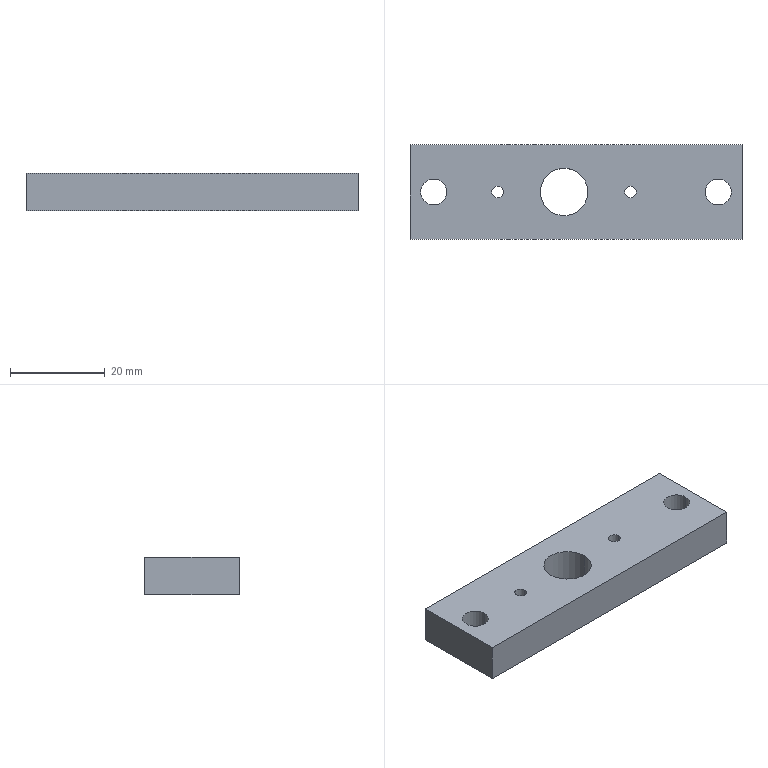Part | STEP file | positioning cylinder plate | 1 solid | 16 faces | box 70 x 20 x 8 mm | volume 10113 mm3 | cylinder 10 | plane 6 | commonest cylinder face diameters 2.5 x4 5.5 x4 10 x2
STEP:
#1=CARTESIAN_POINT('',(0.,0.,0.));
#2=DIRECTION('',(0.,0.,1.));
#3=DIRECTION('',(1.,0.,0.));
#4=AXIS2_PLACEMENT_3D('',#1,#2,#3);
#5=CARTESIAN_POINT('',(-12.75,0.,0.));
#6=VERTEX_POINT('',#5);
#7=CARTESIAN_POINT('',(-12.75,0.,8.));
#8=VERTEX_POINT('',#7);
#9=CARTESIAN_POINT('',(-12.75,0.,8.));
#10=DIRECTION('',(0.,0.,1.));
#11=VECTOR('',#10,1.);
#12=LINE('',#9,#11);
#13=CARTESIAN_POINT('',(-14.,0.,8.));
#14=DIRECTION('',(0.,0.,1.));
#15=DIRECTION('',(1.,0.,0.));
#16=AXIS2_PLACEMENT_3D('',#13,#14,#15);
#17=CYLINDRICAL_SURFACE('',#16,1.25);
#18=CARTESIAN_POINT('',(6.283,0.));
#19=DIRECTION('',(0.,1.));
#20=VECTOR('',#19,1.);
#21=LINE('',#18,#20);
#22=(GEOMETRIC_REPRESENTATION_CONTEXT(2)PARAMETRIC_REPRESENTATION_CONTEXT()REPRESENTATION_CONTEXT('',''));
#23=DEFINITIONAL_REPRESENTATION('',(#21),#22);
#24=PCURVE('',#17,#23);
#25=CARTESIAN_POINT('',(-14.,0.,8.));
#26=DIRECTION('',(0.,0.,1.));
#27=DIRECTION('',(1.,0.,0.));
#28=AXIS2_PLACEMENT_3D('',#25,#26,#27);
#29=CYLINDRICAL_SURFACE('',#28,1.25);
#30=CARTESIAN_POINT('',(0.,0.));
#31=DIRECTION('',(0.,1.));
#32=VECTOR('',#31,1.);
#33=LINE('',#30,#32);
#34=(GEOMETRIC_REPRESENTATION_CONTEXT(2)PARAMETRIC_REPRESENTATION_CONTEXT()REPRESENTATION_CONTEXT('',''));
#35=DEFINITIONAL_REPRESENTATION('',(#33),#34);
#36=PCURVE('',#29,#35);
#37=SURFACE_CURVE('',#12,(#24,#36),.PCURVE_S1.);
#38=EDGE_CURVE('',#6,#8,#37,.T.);
#39=ORIENTED_EDGE('',*,*,#38,.T.);
#40=CARTESIAN_POINT('',(-15.25,0.,8.));
#41=VERTEX_POINT('',#40);
#42=CARTESIAN_POINT('',(-14.,0.,8.));
#43=DIRECTION('',(0.,0.,1.));
#44=DIRECTION('',(1.,0.,0.));
#45=AXIS2_PLACEMENT_3D('',#42,#43,#44);
#46=CIRCLE('',#45,1.25);
#47=CARTESIAN_POINT('',(0.,0.));
#48=DIRECTION('',(1.,0.));
#49=VECTOR('',#48,1.);
#50=LINE('',#47,#49);
#51=(GEOMETRIC_REPRESENTATION_CONTEXT(2)PARAMETRIC_REPRESENTATION_CONTEXT()REPRESENTATION_CONTEXT('',''));
#52=DEFINITIONAL_REPRESENTATION('',(#50),#51);
#53=PCURVE('',#17,#52);
#54=CARTESIAN_POINT('',(37.5,-10.,8.));
#55=DIRECTION('',(0.,0.,1.));
#56=DIRECTION('',(1.,0.,0.));
#57=AXIS2_PLACEMENT_3D('',#54,#55,#56);
#58=PLANE('',#57);
#59=CARTESIAN_POINT('',(-51.5,10.));
#60=DIRECTION('',(1.,0.));
#61=AXIS2_PLACEMENT_2D('',#59,#60);
#62=CIRCLE('',#61,1.25);
#63=(GEOMETRIC_REPRESENTATION_CONTEXT(2)PARAMETRIC_REPRESENTATION_CONTEXT()REPRESENTATION_CONTEXT('',''));
#64=DEFINITIONAL_REPRESENTATION('',(#62),#63);
#65=PCURVE('',#58,#64);
#66=SURFACE_CURVE('',#46,(#53,#65),.PCURVE_S1.);
#67=EDGE_CURVE('',#41,#8,#66,.T.);
#68=ORIENTED_EDGE('',*,*,#67,.F.);
#69=CARTESIAN_POINT('',(-15.25,0.,0.));
#70=VERTEX_POINT('',#69);
#71=CARTESIAN_POINT('',(-15.25,0.,8.));
#72=DIRECTION('',(0.,0.,1.));
#73=VECTOR('',#72,1.);
#74=LINE('',#71,#73);
#75=CARTESIAN_POINT('',(3.142,0.));
#76=DIRECTION('',(0.,1.));
#77=VECTOR('',#76,1.);
#78=LINE('',#75,#77);
#79=(GEOMETRIC_REPRESENTATION_CONTEXT(2)PARAMETRIC_REPRESENTATION_CONTEXT()REPRESENTATION_CONTEXT('',''));
#80=DEFINITIONAL_REPRESENTATION('',(#78),#79);
#81=PCURVE('',#17,#80);
#82=CARTESIAN_POINT('',(3.142,0.));
#83=DIRECTION('',(0.,1.));
#84=VECTOR('',#83,1.);
#85=LINE('',#82,#84);
#86=(GEOMETRIC_REPRESENTATION_CONTEXT(2)PARAMETRIC_REPRESENTATION_CONTEXT()REPRESENTATION_CONTEXT('',''));
#87=DEFINITIONAL_REPRESENTATION('',(#85),#86);
#88=PCURVE('',#29,#87);
#89=SURFACE_CURVE('',#74,(#81,#88),.PCURVE_S1.);
#90=EDGE_CURVE('',#70,#41,#89,.T.);
#91=ORIENTED_EDGE('',*,*,#90,.F.);
#92=CARTESIAN_POINT('',(-14.,0.,0.));
#93=DIRECTION('',(0.,0.,1.));
#94=DIRECTION('',(1.,0.,0.));
#95=AXIS2_PLACEMENT_3D('',#92,#93,#94);
#96=CIRCLE('',#95,1.25);
#97=CARTESIAN_POINT('',(0.,-8.));
#98=DIRECTION('',(1.,0.));
#99=VECTOR('',#98,1.);
#100=LINE('',#97,#99);
#101=(GEOMETRIC_REPRESENTATION_CONTEXT(2)PARAMETRIC_REPRESENTATION_CONTEXT()REPRESENTATION_CONTEXT('',''));
#102=DEFINITIONAL_REPRESENTATION('',(#100),#101);
#103=PCURVE('',#17,#102);
#104=CARTESIAN_POINT('',(37.5,-10.,0.));
#105=DIRECTION('',(0.,0.,1.));
#106=DIRECTION('',(1.,0.,0.));
#107=AXIS2_PLACEMENT_3D('',#104,#105,#106);
#108=PLANE('',#107);
#109=CARTESIAN_POINT('',(-51.5,10.));
#110=DIRECTION('',(1.,0.));
#111=AXIS2_PLACEMENT_2D('',#109,#110);
#112=CIRCLE('',#111,1.25);
#113=(GEOMETRIC_REPRESENTATION_CONTEXT(2)PARAMETRIC_REPRESENTATION_CONTEXT()REPRESENTATION_CONTEXT('',''));
#114=DEFINITIONAL_REPRESENTATION('',(#112),#113);
#115=PCURVE('',#108,#114);
#116=SURFACE_CURVE('',#96,(#103,#115),.PCURVE_S1.);
#117=EDGE_CURVE('',#70,#6,#116,.T.);
#118=ORIENTED_EDGE('',*,*,#117,.T.);
#119=EDGE_LOOP('',(#39,#68,#91,#118));
#120=FACE_BOUND('',#119,.F.);
#121=ADVANCED_FACE('',(#120),#17,.F.);
#122=CARTESIAN_POINT('',(15.25,0.,0.));
#123=VERTEX_POINT('',#122);
#124=CARTESIAN_POINT('',(15.25,0.,8.));
#125=VERTEX_POINT('',#124);
#126=CARTESIAN_POINT('',(15.25,0.,8.));
#127=DIRECTION('',(0.,0.,1.));
#128=VECTOR('',#127,1.);
#129=LINE('',#126,#128);
#130=CARTESIAN_POINT('',(14.,0.,8.));
#131=DIRECTION('',(0.,0.,1.));
#132=DIRECTION('',(1.,0.,0.));
#133=AXIS2_PLACEMENT_3D('',#130,#131,#132);
#134=CYLINDRICAL_SURFACE('',#133,1.25);
#135=CARTESIAN_POINT('',(6.283,0.));
#136=DIRECTION('',(0.,1.));
#137=VECTOR('',#136,1.);
#138=LINE('',#135,#137);
#139=(GEOMETRIC_REPRESENTATION_CONTEXT(2)PARAMETRIC_REPRESENTATION_CONTEXT()REPRESENTATION_CONTEXT('',''));
#140=DEFINITIONAL_REPRESENTATION('',(#138),#139);
#141=PCURVE('',#134,#140);
#142=CARTESIAN_POINT('',(14.,0.,8.));
#143=DIRECTION('',(0.,0.,1.));
#144=DIRECTION('',(1.,0.,0.));
#145=AXIS2_PLACEMENT_3D('',#142,#143,#144);
#146=CYLINDRICAL_SURFACE('',#145,1.25);
#147=CARTESIAN_POINT('',(0.,0.));
#148=DIRECTION('',(0.,1.));
#149=VECTOR('',#148,1.);
#150=LINE('',#147,#149);
#151=(GEOMETRIC_REPRESENTATION_CONTEXT(2)PARAMETRIC_REPRESENTATION_CONTEXT()REPRESENTATION_CONTEXT('',''));
#152=DEFINITIONAL_REPRESENTATION('',(#150),#151);
#153=PCURVE('',#146,#152);
#154=SURFACE_CURVE('',#129,(#141,#153),.PCURVE_S1.);
#155=EDGE_CURVE('',#123,#125,#154,.T.);
#156=ORIENTED_EDGE('',*,*,#155,.T.);
#157=CARTESIAN_POINT('',(12.75,0.,8.));
#158=VERTEX_POINT('',#157);
#159=CARTESIAN_POINT('',(14.,0.,8.));
#160=DIRECTION('',(0.,0.,1.));
#161=DIRECTION('',(1.,0.,0.));
#162=AXIS2_PLACEMENT_3D('',#159,#160,#161);
#163=CIRCLE('',#162,1.25);
#164=CARTESIAN_POINT('',(0.,0.));
#165=DIRECTION('',(1.,0.));
#166=VECTOR('',#165,1.);
#167=LINE('',#164,#166);
#168=(GEOMETRIC_REPRESENTATION_CONTEXT(2)PARAMETRIC_REPRESENTATION_CONTEXT()REPRESENTATION_CONTEXT('',''));
#169=DEFINITIONAL_REPRESENTATION('',(#167),#168);
#170=PCURVE('',#134,#169);
#171=CARTESIAN_POINT('',(-23.5,10.));
#172=DIRECTION('',(1.,0.));
#173=AXIS2_PLACEMENT_2D('',#171,#172);
#174=CIRCLE('',#173,1.25);
#175=(GEOMETRIC_REPRESENTATION_CONTEXT(2)PARAMETRIC_REPRESENTATION_CONTEXT()REPRESENTATION_CONTEXT('',''));
#176=DEFINITIONAL_REPRESENTATION('',(#174),#175);
#177=PCURVE('',#58,#176);
#178=SURFACE_CURVE('',#163,(#170,#177),.PCURVE_S1.);
#179=EDGE_CURVE('',#158,#125,#178,.T.);
#180=ORIENTED_EDGE('',*,*,#179,.F.);
#181=CARTESIAN_POINT('',(12.75,0.,0.));
#182=VERTEX_POINT('',#181);
#183=CARTESIAN_POINT('',(12.75,0.,8.));
#184=DIRECTION('',(0.,0.,1.));
#185=VECTOR('',#184,1.);
#186=LINE('',#183,#185);
#187=CARTESIAN_POINT('',(3.142,0.));
#188=DIRECTION('',(0.,1.));
#189=VECTOR('',#188,1.);
#190=LINE('',#187,#189);
#191=(GEOMETRIC_REPRESENTATION_CONTEXT(2)PARAMETRIC_REPRESENTATION_CONTEXT()REPRESENTATION_CONTEXT('',''));
#192=DEFINITIONAL_REPRESENTATION('',(#190),#191);
#193=PCURVE('',#134,#192);
#194=CARTESIAN_POINT('',(3.142,0.));
#195=DIRECTION('',(0.,1.));
#196=VECTOR('',#195,1.);
#197=LINE('',#194,#196);
#198=(GEOMETRIC_REPRESENTATION_CONTEXT(2)PARAMETRIC_REPRESENTATION_CONTEXT()REPRESENTATION_CONTEXT('',''));
#199=DEFINITIONAL_REPRESENTATION('',(#197),#198);
#200=PCURVE('',#146,#199);
#201=SURFACE_CURVE('',#186,(#193,#200),.PCURVE_S1.);
#202=EDGE_CURVE('',#182,#158,#201,.T.);
#203=ORIENTED_EDGE('',*,*,#202,.F.);
#204=CARTESIAN_POINT('',(14.,0.,0.));
#205=DIRECTION('',(0.,0.,1.));
#206=DIRECTION('',(1.,0.,0.));
#207=AXIS2_PLACEMENT_3D('',#204,#205,#206);
#208=CIRCLE('',#207,1.25);
#209=CARTESIAN_POINT('',(0.,-8.));
#210=DIRECTION('',(1.,0.));
#211=VECTOR('',#210,1.);
#212=LINE('',#209,#211);
#213=(GEOMETRIC_REPRESENTATION_CONTEXT(2)PARAMETRIC_REPRESENTATION_CONTEXT()REPRESENTATION_CONTEXT('',''));
#214=DEFINITIONAL_REPRESENTATION('',(#212),#213);
#215=PCURVE('',#134,#214);
#216=CARTESIAN_POINT('',(-23.5,10.));
#217=DIRECTION('',(1.,0.));
#218=AXIS2_PLACEMENT_2D('',#216,#217);
#219=CIRCLE('',#218,1.25);
#220=(GEOMETRIC_REPRESENTATION_CONTEXT(2)PARAMETRIC_REPRESENTATION_CONTEXT()REPRESENTATION_CONTEXT('',''));
#221=DEFINITIONAL_REPRESENTATION('',(#219),#220);
#222=PCURVE('',#108,#221);
#223=SURFACE_CURVE('',#208,(#215,#222),.PCURVE_S1.);
#224=EDGE_CURVE('',#182,#123,#223,.T.);
#225=ORIENTED_EDGE('',*,*,#224,.T.);
#226=EDGE_LOOP('',(#156,#180,#203,#225));
#227=FACE_BOUND('',#226,.F.);
#228=ADVANCED_FACE('',(#227),#134,.F.);
#229=CARTESIAN_POINT('',(-5.,0.,8.));
#230=VERTEX_POINT('',#229);
#231=CARTESIAN_POINT('',(-5.,0.,0.));
#232=VERTEX_POINT('',#231);
#233=CARTESIAN_POINT('',(-5.,0.,8.));
#234=DIRECTION('',(0.,0.,-1.));
#235=VECTOR('',#234,1.);
#236=LINE('',#233,#235);
#237=CARTESIAN_POINT('',(0.,0.,8.));
#238=DIRECTION('',(0.,0.,-1.));
#239=DIRECTION('',(-1.,0.,0.));
#240=AXIS2_PLACEMENT_3D('',#237,#238,#239);
#241=CYLINDRICAL_SURFACE('',#240,5.);
#242=CARTESIAN_POINT('',(6.283,0.));
#243=DIRECTION('',(0.,1.));
#244=VECTOR('',#243,1.);
#245=LINE('',#242,#244);
#246=(GEOMETRIC_REPRESENTATION_CONTEXT(2)PARAMETRIC_REPRESENTATION_CONTEXT()REPRESENTATION_CONTEXT('',''));
#247=DEFINITIONAL_REPRESENTATION('',(#245),#246);
#248=PCURVE('',#241,#247);
#249=CARTESIAN_POINT('',(0.,0.,8.));
#250=DIRECTION('',(0.,0.,-1.));
#251=DIRECTION('',(-1.,0.,0.));
#252=AXIS2_PLACEMENT_3D('',#249,#250,#251);
#253=CYLINDRICAL_SURFACE('',#252,5.);
#254=CARTESIAN_POINT('',(0.,0.));
#255=DIRECTION('',(0.,1.));
#256=VECTOR('',#255,1.);
#257=LINE('',#254,#256);
#258=(GEOMETRIC_REPRESENTATION_CONTEXT(2)PARAMETRIC_REPRESENTATION_CONTEXT()REPRESENTATION_CONTEXT('',''));
#259=DEFINITIONAL_REPRESENTATION('',(#257),#258);
#260=PCURVE('',#253,#259);
#261=SURFACE_CURVE('',#236,(#248,#260),.PCURVE_S1.);
#262=EDGE_CURVE('',#230,#232,#261,.T.);
#263=ORIENTED_EDGE('',*,*,#262,.T.);
#264=CARTESIAN_POINT('',(5.,0.,0.));
#265=VERTEX_POINT('',#264);
#266=CARTESIAN_POINT('',(0.,0.,0.));
#267=DIRECTION('',(0.,0.,1.));
#268=DIRECTION('',(1.,0.,0.));
#269=AXIS2_PLACEMENT_3D('',#266,#267,#268);
#270=CIRCLE('',#269,5.);
#271=CARTESIAN_POINT('',(9.425,8.));
#272=DIRECTION('',(-1.,0.));
#273=VECTOR('',#272,1.);
#274=LINE('',#271,#273);
#275=(GEOMETRIC_REPRESENTATION_CONTEXT(2)PARAMETRIC_REPRESENTATION_CONTEXT()REPRESENTATION_CONTEXT('',''));
#276=DEFINITIONAL_REPRESENTATION('',(#274),#275);
#277=PCURVE('',#241,#276);
#278=CARTESIAN_POINT('',(-37.5,10.));
#279=DIRECTION('',(1.,0.));
#280=AXIS2_PLACEMENT_2D('',#278,#279);
#281=CIRCLE('',#280,5.);
#282=(GEOMETRIC_REPRESENTATION_CONTEXT(2)PARAMETRIC_REPRESENTATION_CONTEXT()REPRESENTATION_CONTEXT('',''));
#283=DEFINITIONAL_REPRESENTATION('',(#281),#282);
#284=PCURVE('',#108,#283);
#285=SURFACE_CURVE('',#270,(#277,#284),.PCURVE_S1.);
#286=EDGE_CURVE('',#232,#265,#285,.T.);
#287=ORIENTED_EDGE('',*,*,#286,.T.);
#288=CARTESIAN_POINT('',(5.,0.,8.));
#289=VERTEX_POINT('',#288);
#290=CARTESIAN_POINT('',(5.,0.,8.));
#291=DIRECTION('',(0.,0.,-1.));
#292=VECTOR('',#291,1.);
#293=LINE('',#290,#292);
#294=CARTESIAN_POINT('',(3.142,0.));
#295=DIRECTION('',(0.,1.));
#296=VECTOR('',#295,1.);
#297=LINE('',#294,#296);
#298=(GEOMETRIC_REPRESENTATION_CONTEXT(2)PARAMETRIC_REPRESENTATION_CONTEXT()REPRESENTATION_CONTEXT('',''));
#299=DEFINITIONAL_REPRESENTATION('',(#297),#298);
#300=PCURVE('',#241,#299);
#301=CARTESIAN_POINT('',(3.142,0.));
#302=DIRECTION('',(0.,1.));
#303=VECTOR('',#302,1.);
#304=LINE('',#301,#303);
#305=(GEOMETRIC_REPRESENTATION_CONTEXT(2)PARAMETRIC_REPRESENTATION_CONTEXT()REPRESENTATION_CONTEXT('',''));
#306=DEFINITIONAL_REPRESENTATION('',(#304),#305);
#307=PCURVE('',#253,#306);
#308=SURFACE_CURVE('',#293,(#300,#307),.PCURVE_S1.);
#309=EDGE_CURVE('',#289,#265,#308,.T.);
#310=ORIENTED_EDGE('',*,*,#309,.F.);
#311=CARTESIAN_POINT('',(0.,0.,8.));
#312=DIRECTION('',(0.,0.,1.));
#313=DIRECTION('',(1.,0.,0.));
#314=AXIS2_PLACEMENT_3D('',#311,#312,#313);
#315=CIRCLE('',#314,5.);
#316=CARTESIAN_POINT('',(9.425,0.));
#317=DIRECTION('',(-1.,0.));
#318=VECTOR('',#317,1.);
#319=LINE('',#316,#318);
#320=(GEOMETRIC_REPRESENTATION_CONTEXT(2)PARAMETRIC_REPRESENTATION_CONTEXT()REPRESENTATION_CONTEXT('',''));
#321=DEFINITIONAL_REPRESENTATION('',(#319),#320);
#322=PCURVE('',#241,#321);
#323=CARTESIAN_POINT('',(-37.5,10.));
#324=DIRECTION('',(1.,0.));
#325=AXIS2_PLACEMENT_2D('',#323,#324);
#326=CIRCLE('',#325,5.);
#327=(GEOMETRIC_REPRESENTATION_CONTEXT(2)PARAMETRIC_REPRESENTATION_CONTEXT()REPRESENTATION_CONTEXT('',''));
#328=DEFINITIONAL_REPRESENTATION('',(#326),#327);
#329=PCURVE('',#58,#328);
#330=SURFACE_CURVE('',#315,(#322,#329),.PCURVE_S1.);
#331=EDGE_CURVE('',#230,#289,#330,.T.);
#332=ORIENTED_EDGE('',*,*,#331,.F.);
#333=EDGE_LOOP('',(#263,#287,#310,#332));
#334=FACE_BOUND('',#333,.F.);
#335=ADVANCED_FACE('',(#334),#241,.F.);
#336=CARTESIAN_POINT('',(-30.25,0.,8.));
#337=VERTEX_POINT('',#336);
#338=CARTESIAN_POINT('',(-30.25,0.,0.));
#339=VERTEX_POINT('',#338);
#340=CARTESIAN_POINT('',(-30.25,0.,8.));
#341=DIRECTION('',(0.,0.,-1.));
#342=VECTOR('',#341,1.);
#343=LINE('',#340,#342);
#344=CARTESIAN_POINT('',(-27.5,0.,8.));
#345=DIRECTION('',(0.,0.,-1.));
#346=DIRECTION('',(-1.,0.,0.));
#347=AXIS2_PLACEMENT_3D('',#344,#345,#346);
#348=CYLINDRICAL_SURFACE('',#347,2.75);
#349=CARTESIAN_POINT('',(6.283,0.));
#350=DIRECTION('',(0.,1.));
#351=VECTOR('',#350,1.);
#352=LINE('',#349,#351);
#353=(GEOMETRIC_REPRESENTATION_CONTEXT(2)PARAMETRIC_REPRESENTATION_CONTEXT()REPRESENTATION_CONTEXT('',''));
#354=DEFINITIONAL_REPRESENTATION('',(#352),#353);
#355=PCURVE('',#348,#354);
#356=CARTESIAN_POINT('',(-27.5,0.,8.));
#357=DIRECTION('',(0.,0.,-1.));
#358=DIRECTION('',(-1.,0.,0.));
#359=AXIS2_PLACEMENT_3D('',#356,#357,#358);
#360=CYLINDRICAL_SURFACE('',#359,2.75);
#361=CARTESIAN_POINT('',(0.,0.));
#362=DIRECTION('',(0.,1.));
#363=VECTOR('',#362,1.);
#364=LINE('',#361,#363);
#365=(GEOMETRIC_REPRESENTATION_CONTEXT(2)PARAMETRIC_REPRESENTATION_CONTEXT()REPRESENTATION_CONTEXT('',''));
#366=DEFINITIONAL_REPRESENTATION('',(#364),#365);
#367=PCURVE('',#360,#366);
#368=SURFACE_CURVE('',#343,(#355,#367),.PCURVE_S1.);
#369=EDGE_CURVE('',#337,#339,#368,.T.);
#370=ORIENTED_EDGE('',*,*,#369,.T.);
#371=CARTESIAN_POINT('',(-24.75,0.,0.));
#372=VERTEX_POINT('',#371);
#373=CARTESIAN_POINT('',(-27.5,0.,0.));
#374=DIRECTION('',(0.,0.,1.));
#375=DIRECTION('',(1.,0.,0.));
#376=AXIS2_PLACEMENT_3D('',#373,#374,#375);
#377=CIRCLE('',#376,2.75);
#378=CARTESIAN_POINT('',(9.425,8.));
#379=DIRECTION('',(-1.,0.));
#380=VECTOR('',#379,1.);
#381=LINE('',#378,#380);
#382=(GEOMETRIC_REPRESENTATION_CONTEXT(2)PARAMETRIC_REPRESENTATION_CONTEXT()REPRESENTATION_CONTEXT('',''));
#383=DEFINITIONAL_REPRESENTATION('',(#381),#382);
#384=PCURVE('',#348,#383);
#385=CARTESIAN_POINT('',(-65.,10.));
#386=DIRECTION('',(1.,0.));
#387=AXIS2_PLACEMENT_2D('',#385,#386);
#388=CIRCLE('',#387,2.75);
#389=(GEOMETRIC_REPRESENTATION_CONTEXT(2)PARAMETRIC_REPRESENTATION_CONTEXT()REPRESENTATION_CONTEXT('',''));
#390=DEFINITIONAL_REPRESENTATION('',(#388),#389);
#391=PCURVE('',#108,#390);
#392=SURFACE_CURVE('',#377,(#384,#391),.PCURVE_S1.);
#393=EDGE_CURVE('',#339,#372,#392,.T.);
#394=ORIENTED_EDGE('',*,*,#393,.T.);
#395=CARTESIAN_POINT('',(-24.75,0.,8.));
#396=VERTEX_POINT('',#395);
#397=CARTESIAN_POINT('',(-24.75,0.,8.));
#398=DIRECTION('',(0.,0.,-1.));
#399=VECTOR('',#398,1.);
#400=LINE('',#397,#399);
#401=CARTESIAN_POINT('',(3.142,0.));
#402=DIRECTION('',(0.,1.));
#403=VECTOR('',#402,1.);
#404=LINE('',#401,#403);
#405=(GEOMETRIC_REPRESENTATION_CONTEXT(2)PARAMETRIC_REPRESENTATION_CONTEXT()REPRESENTATION_CONTEXT('',''));
#406=DEFINITIONAL_REPRESENTATION('',(#404),#405);
#407=PCURVE('',#348,#406);
#408=CARTESIAN_POINT('',(3.142,0.));
#409=DIRECTION('',(0.,1.));
#410=VECTOR('',#409,1.);
#411=LINE('',#408,#410);
#412=(GEOMETRIC_REPRESENTATION_CONTEXT(2)PARAMETRIC_REPRESENTATION_CONTEXT()REPRESENTATION_CONTEXT('',''));
#413=DEFINITIONAL_REPRESENTATION('',(#411),#412);
#414=PCURVE('',#360,#413);
#415=SURFACE_CURVE('',#400,(#407,#414),.PCURVE_S1.);
#416=EDGE_CURVE('',#396,#372,#415,.T.);
#417=ORIENTED_EDGE('',*,*,#416,.F.);
#418=CARTESIAN_POINT('',(-27.5,0.,8.));
#419=DIRECTION('',(0.,0.,1.));
#420=DIRECTION('',(1.,0.,0.));
#421=AXIS2_PLACEMENT_3D('',#418,#419,#420);
#422=CIRCLE('',#421,2.75);
#423=CARTESIAN_POINT('',(9.425,0.));
#424=DIRECTION('',(-1.,0.));
#425=VECTOR('',#424,1.);
#426=LINE('',#423,#425);
#427=(GEOMETRIC_REPRESENTATION_CONTEXT(2)PARAMETRIC_REPRESENTATION_CONTEXT()REPRESENTATION_CONTEXT('',''));
#428=DEFINITIONAL_REPRESENTATION('',(#426),#427);
#429=PCURVE('',#348,#428);
#430=CARTESIAN_POINT('',(-65.,10.));
#431=DIRECTION('',(1.,0.));
#432=AXIS2_PLACEMENT_2D('',#430,#431);
#433=CIRCLE('',#432,2.75);
#434=(GEOMETRIC_REPRESENTATION_CONTEXT(2)PARAMETRIC_REPRESENTATION_CONTEXT()REPRESENTATION_CONTEXT('',''));
#435=DEFINITIONAL_REPRESENTATION('',(#433),#434);
#436=PCURVE('',#58,#435);
#437=SURFACE_CURVE('',#422,(#429,#436),.PCURVE_S1.);
#438=EDGE_CURVE('',#337,#396,#437,.T.);
#439=ORIENTED_EDGE('',*,*,#438,.F.);
#440=EDGE_LOOP('',(#370,#394,#417,#439));
#441=FACE_BOUND('',#440,.F.);
#442=ADVANCED_FACE('',(#441),#348,.F.);
#443=CARTESIAN_POINT('',(29.75,0.,8.));
#444=VERTEX_POINT('',#443);
#445=CARTESIAN_POINT('',(29.75,0.,0.));
#446=VERTEX_POINT('',#445);
#447=CARTESIAN_POINT('',(29.75,0.,8.));
#448=DIRECTION('',(0.,0.,-1.));
#449=VECTOR('',#448,1.);
#450=LINE('',#447,#449);
#451=CARTESIAN_POINT('',(32.5,0.,8.));
#452=DIRECTION('',(0.,0.,-1.));
#453=DIRECTION('',(-1.,0.,0.));
#454=AXIS2_PLACEMENT_3D('',#451,#452,#453);
#455=CYLINDRICAL_SURFACE('',#454,2.75);
#456=CARTESIAN_POINT('',(6.283,0.));
#457=DIRECTION('',(0.,1.));
#458=VECTOR('',#457,1.);
#459=LINE('',#456,#458);
#460=(GEOMETRIC_REPRESENTATION_CONTEXT(2)PARAMETRIC_REPRESENTATION_CONTEXT()REPRESENTATION_CONTEXT('',''));
#461=DEFINITIONAL_REPRESENTATION('',(#459),#460);
#462=PCURVE('',#455,#461);
#463=CARTESIAN_POINT('',(32.5,0.,8.));
#464=DIRECTION('',(0.,0.,-1.));
#465=DIRECTION('',(-1.,0.,0.));
#466=AXIS2_PLACEMENT_3D('',#463,#464,#465);
#467=CYLINDRICAL_SURFACE('',#466,2.75);
#468=CARTESIAN_POINT('',(0.,0.));
#469=DIRECTION('',(0.,1.));
#470=VECTOR('',#469,1.);
#471=LINE('',#468,#470);
#472=(GEOMETRIC_REPRESENTATION_CONTEXT(2)PARAMETRIC_REPRESENTATION_CONTEXT()REPRESENTATION_CONTEXT('',''));
#473=DEFINITIONAL_REPRESENTATION('',(#471),#472);
#474=PCURVE('',#467,#473);
#475=SURFACE_CURVE('',#450,(#462,#474),.PCURVE_S1.);
#476=EDGE_CURVE('',#444,#446,#475,.T.);
#477=ORIENTED_EDGE('',*,*,#476,.T.);
#478=CARTESIAN_POINT('',(35.25,0.,0.));
#479=VERTEX_POINT('',#478);
#480=CARTESIAN_POINT('',(32.5,0.,0.));
#481=DIRECTION('',(0.,0.,1.));
#482=DIRECTION('',(1.,0.,0.));
#483=AXIS2_PLACEMENT_3D('',#480,#481,#482);
#484=CIRCLE('',#483,2.75);
#485=CARTESIAN_POINT('',(9.425,8.));
#486=DIRECTION('',(-1.,0.));
#487=VECTOR('',#486,1.);
#488=LINE('',#485,#487);
#489=(GEOMETRIC_REPRESENTATION_CONTEXT(2)PARAMETRIC_REPRESENTATION_CONTEXT()REPRESENTATION_CONTEXT('',''));
#490=DEFINITIONAL_REPRESENTATION('',(#488),#489);
#491=PCURVE('',#455,#490);
#492=CARTESIAN_POINT('',(-5.,10.));
#493=DIRECTION('',(1.,0.));
#494=AXIS2_PLACEMENT_2D('',#492,#493);
#495=CIRCLE('',#494,2.75);
#496=(GEOMETRIC_REPRESENTATION_CONTEXT(2)PARAMETRIC_REPRESENTATION_CONTEXT()REPRESENTATION_CONTEXT('',''));
#497=DEFINITIONAL_REPRESENTATION('',(#495),#496);
#498=PCURVE('',#108,#497);
#499=SURFACE_CURVE('',#484,(#491,#498),.PCURVE_S1.);
#500=EDGE_CURVE('',#446,#479,#499,.T.);
#501=ORIENTED_EDGE('',*,*,#500,.T.);
#502=CARTESIAN_POINT('',(35.25,0.,8.));
#503=VERTEX_POINT('',#502);
#504=CARTESIAN_POINT('',(35.25,0.,8.));
#505=DIRECTION('',(0.,0.,-1.));
#506=VECTOR('',#505,1.);
#507=LINE('',#504,#506);
#508=CARTESIAN_POINT('',(3.142,0.));
#509=DIRECTION('',(0.,1.));
#510=VECTOR('',#509,1.);
#511=LINE('',#508,#510);
#512=(GEOMETRIC_REPRESENTATION_CONTEXT(2)PARAMETRIC_REPRESENTATION_CONTEXT()REPRESENTATION_CONTEXT('',''));
#513=DEFINITIONAL_REPRESENTATION('',(#511),#512);
#514=PCURVE('',#455,#513);
#515=CARTESIAN_POINT('',(3.142,0.));
#516=DIRECTION('',(0.,1.));
#517=VECTOR('',#516,1.);
#518=LINE('',#515,#517);
#519=(GEOMETRIC_REPRESENTATION_CONTEXT(2)PARAMETRIC_REPRESENTATION_CONTEXT()REPRESENTATION_CONTEXT('',''));
#520=DEFINITIONAL_REPRESENTATION('',(#518),#519);
#521=PCURVE('',#467,#520);
#522=SURFACE_CURVE('',#507,(#514,#521),.PCURVE_S1.);
#523=EDGE_CURVE('',#503,#479,#522,.T.);
#524=ORIENTED_EDGE('',*,*,#523,.F.);
#525=CARTESIAN_POINT('',(32.5,0.,8.));
#526=DIRECTION('',(0.,0.,1.));
#527=DIRECTION('',(1.,0.,0.));
#528=AXIS2_PLACEMENT_3D('',#525,#526,#527);
#529=CIRCLE('',#528,2.75);
#530=CARTESIAN_POINT('',(9.425,0.));
#531=DIRECTION('',(-1.,0.));
#532=VECTOR('',#531,1.);
#533=LINE('',#530,#532);
#534=(GEOMETRIC_REPRESENTATION_CONTEXT(2)PARAMETRIC_REPRESENTATION_CONTEXT()REPRESENTATION_CONTEXT('',''));
#535=DEFINITIONAL_REPRESENTATION('',(#533),#534);
#536=PCURVE('',#455,#535);
#537=CARTESIAN_POINT('',(-5.,10.));
#538=DIRECTION('',(1.,0.));
#539=AXIS2_PLACEMENT_2D('',#537,#538);
#540=CIRCLE('',#539,2.75);
#541=(GEOMETRIC_REPRESENTATION_CONTEXT(2)PARAMETRIC_REPRESENTATION_CONTEXT()REPRESENTATION_CONTEXT('',''));
#542=DEFINITIONAL_REPRESENTATION('',(#540),#541);
#543=PCURVE('',#58,#542);
#544=SURFACE_CURVE('',#529,(#536,#543),.PCURVE_S1.);
#545=EDGE_CURVE('',#444,#503,#544,.T.);
#546=ORIENTED_EDGE('',*,*,#545,.F.);
#547=EDGE_LOOP('',(#477,#501,#524,#546));
#548=FACE_BOUND('',#547,.F.);
#549=ADVANCED_FACE('',(#548),#455,.F.);
#550=CARTESIAN_POINT('',(-14.,0.,8.));
#551=DIRECTION('',(0.,0.,1.));
#552=DIRECTION('',(1.,0.,0.));
#553=AXIS2_PLACEMENT_3D('',#550,#551,#552);
#554=CIRCLE('',#553,1.25);
#555=CARTESIAN_POINT('',(-51.5,10.));
#556=DIRECTION('',(1.,0.));
#557=AXIS2_PLACEMENT_2D('',#555,#556);
#558=CIRCLE('',#557,1.25);
#559=(GEOMETRIC_REPRESENTATION_CONTEXT(2)PARAMETRIC_REPRESENTATION_CONTEXT()REPRESENTATION_CONTEXT('',''));
#560=DEFINITIONAL_REPRESENTATION('',(#558),#559);
#561=PCURVE('',#58,#560);
#562=CARTESIAN_POINT('',(0.,0.));
#563=DIRECTION('',(1.,0.));
#564=VECTOR('',#563,1.);
#565=LINE('',#562,#564);
#566=(GEOMETRIC_REPRESENTATION_CONTEXT(2)PARAMETRIC_REPRESENTATION_CONTEXT()REPRESENTATION_CONTEXT('',''));
#567=DEFINITIONAL_REPRESENTATION('',(#565),#566);
#568=PCURVE('',#29,#567);
#569=SURFACE_CURVE('',#554,(#561,#568),.PCURVE_S1.);
#570=EDGE_CURVE('',#8,#41,#569,.T.);
#571=ORIENTED_EDGE('',*,*,#570,.F.);
#572=ORIENTED_EDGE('',*,*,#67,.F.);
#573=EDGE_LOOP('',(#571,#572));
#574=FACE_BOUND('',#573,.T.);
#575=CARTESIAN_POINT('',(14.,0.,8.));
#576=DIRECTION('',(0.,0.,1.));
#577=DIRECTION('',(1.,0.,0.));
#578=AXIS2_PLACEMENT_3D('',#575,#576,#577);
#579=CIRCLE('',#578,1.25);
#580=CARTESIAN_POINT('',(-23.5,10.));
#581=DIRECTION('',(1.,0.));
#582=AXIS2_PLACEMENT_2D('',#580,#581);
#583=CIRCLE('',#582,1.25);
#584=(GEOMETRIC_REPRESENTATION_CONTEXT(2)PARAMETRIC_REPRESENTATION_CONTEXT()REPRESENTATION_CONTEXT('',''));
#585=DEFINITIONAL_REPRESENTATION('',(#583),#584);
#586=PCURVE('',#58,#585);
#587=CARTESIAN_POINT('',(0.,0.));
#588=DIRECTION('',(1.,0.));
#589=VECTOR('',#588,1.);
#590=LINE('',#587,#589);
#591=(GEOMETRIC_REPRESENTATION_CONTEXT(2)PARAMETRIC_REPRESENTATION_CONTEXT()REPRESENTATION_CONTEXT('',''));
#592=DEFINITIONAL_REPRESENTATION('',(#590),#591);
#593=PCURVE('',#146,#592);
#594=SURFACE_CURVE('',#579,(#586,#593),.PCURVE_S1.);
#595=EDGE_CURVE('',#125,#158,#594,.T.);
#596=ORIENTED_EDGE('',*,*,#595,.F.);
#597=ORIENTED_EDGE('',*,*,#179,.F.);
#598=EDGE_LOOP('',(#596,#597));
#599=FACE_BOUND('',#598,.T.);
#600=ORIENTED_EDGE('',*,*,#438,.F.);
#601=CARTESIAN_POINT('',(-27.5,0.,8.));
#602=DIRECTION('',(0.,0.,1.));
#603=DIRECTION('',(1.,0.,0.));
#604=AXIS2_PLACEMENT_3D('',#601,#602,#603);
#605=CIRCLE('',#604,2.75);
#606=CARTESIAN_POINT('',(-65.,10.));
#607=DIRECTION('',(1.,0.));
#608=AXIS2_PLACEMENT_2D('',#606,#607);
#609=CIRCLE('',#608,2.75);
#610=(GEOMETRIC_REPRESENTATION_CONTEXT(2)PARAMETRIC_REPRESENTATION_CONTEXT()REPRESENTATION_CONTEXT('',''));
#611=DEFINITIONAL_REPRESENTATION('',(#609),#610);
#612=PCURVE('',#58,#611);
#613=CARTESIAN_POINT('',(3.142,0.));
#614=DIRECTION('',(-1.,0.));
#615=VECTOR('',#614,1.);
#616=LINE('',#613,#615);
#617=(GEOMETRIC_REPRESENTATION_CONTEXT(2)PARAMETRIC_REPRESENTATION_CONTEXT()REPRESENTATION_CONTEXT('',''));
#618=DEFINITIONAL_REPRESENTATION('',(#616),#617);
#619=PCURVE('',#360,#618);
#620=SURFACE_CURVE('',#605,(#612,#619),.PCURVE_S1.);
#621=EDGE_CURVE('',#396,#337,#620,.T.);
#622=ORIENTED_EDGE('',*,*,#621,.F.);
#623=EDGE_LOOP('',(#600,#622));
#624=FACE_BOUND('',#623,.T.);
#625=CARTESIAN_POINT('',(37.5,-10.,8.));
#626=VERTEX_POINT('',#625);
#627=CARTESIAN_POINT('',(37.5,10.,8.));
#628=VERTEX_POINT('',#627);
#629=CARTESIAN_POINT('',(37.5,10.,8.));
#630=DIRECTION('',(0.,1.,0.));
#631=VECTOR('',#630,1.);
#632=LINE('',#629,#631);
#633=CARTESIAN_POINT('',(0.,20.));
#634=DIRECTION('',(0.,1.));
#635=VECTOR('',#634,1.);
#636=LINE('',#633,#635);
#637=(GEOMETRIC_REPRESENTATION_CONTEXT(2)PARAMETRIC_REPRESENTATION_CONTEXT()REPRESENTATION_CONTEXT('',''));
#638=DEFINITIONAL_REPRESENTATION('',(#636),#637);
#639=PCURVE('',#58,#638);
#640=CARTESIAN_POINT('',(37.5,10.,8.));
#641=DIRECTION('',(-1.,0.,0.));
#642=DIRECTION('',(0.,-1.,0.));
#643=AXIS2_PLACEMENT_3D('',#640,#641,#642);
#644=PLANE('',#643);
#645=CARTESIAN_POINT('',(0.,0.));
#646=DIRECTION('',(-1.,0.));
#647=VECTOR('',#646,1.);
#648=LINE('',#645,#647);
#649=(GEOMETRIC_REPRESENTATION_CONTEXT(2)PARAMETRIC_REPRESENTATION_CONTEXT()REPRESENTATION_CONTEXT('',''));
#650=DEFINITIONAL_REPRESENTATION('',(#648),#649);
#651=PCURVE('',#644,#650);
#652=SURFACE_CURVE('',#632,(#639,#651),.PCURVE_S1.);
#653=EDGE_CURVE('',#626,#628,#652,.T.);
#654=ORIENTED_EDGE('',*,*,#653,.T.);
#655=CARTESIAN_POINT('',(-32.5,10.,8.));
#656=VERTEX_POINT('',#655);
#657=CARTESIAN_POINT('',(-32.5,10.,8.));
#658=DIRECTION('',(-1.,0.,0.));
#659=VECTOR('',#658,1.);
#660=LINE('',#657,#659);
#661=CARTESIAN_POINT('',(-70.,20.));
#662=DIRECTION('',(-1.,0.));
#663=VECTOR('',#662,1.);
#664=LINE('',#661,#663);
#665=(GEOMETRIC_REPRESENTATION_CONTEXT(2)PARAMETRIC_REPRESENTATION_CONTEXT()REPRESENTATION_CONTEXT('',''));
#666=DEFINITIONAL_REPRESENTATION('',(#664),#665);
#667=PCURVE('',#58,#666);
#668=CARTESIAN_POINT('',(-32.5,10.,8.));
#669=DIRECTION('',(0.,-1.,0.));
#670=DIRECTION('',(1.,0.,0.));
#671=AXIS2_PLACEMENT_3D('',#668,#669,#670);
#672=PLANE('',#671);
#673=CARTESIAN_POINT('',(0.,0.));
#674=DIRECTION('',(-1.,0.));
#675=VECTOR('',#674,1.);
#676=LINE('',#673,#675);
#677=(GEOMETRIC_REPRESENTATION_CONTEXT(2)PARAMETRIC_REPRESENTATION_CONTEXT()REPRESENTATION_CONTEXT('',''));
#678=DEFINITIONAL_REPRESENTATION('',(#676),#677);
#679=PCURVE('',#672,#678);
#680=SURFACE_CURVE('',#660,(#667,#679),.PCURVE_S1.);
#681=EDGE_CURVE('',#628,#656,#680,.T.);
#682=ORIENTED_EDGE('',*,*,#681,.T.);
#683=CARTESIAN_POINT('',(-32.5,-10.,8.));
#684=VERTEX_POINT('',#683);
#685=CARTESIAN_POINT('',(-32.5,10.,8.));
#686=DIRECTION('',(0.,-1.,0.));
#687=VECTOR('',#686,1.);
#688=LINE('',#685,#687);
#689=CARTESIAN_POINT('',(-70.,20.));
#690=DIRECTION('',(0.,-1.));
#691=VECTOR('',#690,1.);
#692=LINE('',#689,#691);
#693=(GEOMETRIC_REPRESENTATION_CONTEXT(2)PARAMETRIC_REPRESENTATION_CONTEXT()REPRESENTATION_CONTEXT('',''));
#694=DEFINITIONAL_REPRESENTATION('',(#692),#693);
#695=PCURVE('',#58,#694);
#696=CARTESIAN_POINT('',(-32.5,10.,8.));
#697=DIRECTION('',(1.,0.,0.));
#698=DIRECTION('',(0.,1.,0.));
#699=AXIS2_PLACEMENT_3D('',#696,#697,#698);
#700=PLANE('',#699);
#701=CARTESIAN_POINT('',(0.,0.));
#702=DIRECTION('',(-1.,0.));
#703=VECTOR('',#702,1.);
#704=LINE('',#701,#703);
#705=(GEOMETRIC_REPRESENTATION_CONTEXT(2)PARAMETRIC_REPRESENTATION_CONTEXT()REPRESENTATION_CONTEXT('',''));
#706=DEFINITIONAL_REPRESENTATION('',(#704),#705);
#707=PCURVE('',#700,#706);
#708=SURFACE_CURVE('',#688,(#695,#707),.PCURVE_S1.);
#709=EDGE_CURVE('',#656,#684,#708,.T.);
#710=ORIENTED_EDGE('',*,*,#709,.T.);
#711=CARTESIAN_POINT('',(-32.5,-10.,8.));
#712=DIRECTION('',(1.,0.,0.));
#713=VECTOR('',#712,1.);
#714=LINE('',#711,#713);
#715=CARTESIAN_POINT('',(-70.,0.));
#716=DIRECTION('',(1.,0.));
#717=VECTOR('',#716,1.);
#718=LINE('',#715,#717);
#719=(GEOMETRIC_REPRESENTATION_CONTEXT(2)PARAMETRIC_REPRESENTATION_CONTEXT()REPRESENTATION_CONTEXT('',''));
#720=DEFINITIONAL_REPRESENTATION('',(#718),#719);
#721=PCURVE('',#58,#720);
#722=CARTESIAN_POINT('',(-32.5,-10.,8.));
#723=DIRECTION('',(0.,1.,0.));
#724=DIRECTION('',(0.,0.,1.));
#725=AXIS2_PLACEMENT_3D('',#722,#723,#724);
#726=PLANE('',#725);
#727=CARTESIAN_POINT('',(0.,0.));
#728=DIRECTION('',(0.,1.));
#729=VECTOR('',#728,1.);
#730=LINE('',#727,#729);
#731=(GEOMETRIC_REPRESENTATION_CONTEXT(2)PARAMETRIC_REPRESENTATION_CONTEXT()REPRESENTATION_CONTEXT('',''));
#732=DEFINITIONAL_REPRESENTATION('',(#730),#731);
#733=PCURVE('',#726,#732);
#734=SURFACE_CURVE('',#714,(#721,#733),.PCURVE_S1.);
#735=EDGE_CURVE('',#684,#626,#734,.T.);
#736=ORIENTED_EDGE('',*,*,#735,.T.);
#737=EDGE_LOOP('',(#654,#682,#710,#736));
#738=FACE_BOUND('',#737,.T.);
#739=ORIENTED_EDGE('',*,*,#545,.F.);
#740=CARTESIAN_POINT('',(32.5,0.,8.));
#741=DIRECTION('',(0.,0.,1.));
#742=DIRECTION('',(1.,0.,0.));
#743=AXIS2_PLACEMENT_3D('',#740,#741,#742);
#744=CIRCLE('',#743,2.75);
#745=CARTESIAN_POINT('',(-5.,10.));
#746=DIRECTION('',(1.,0.));
#747=AXIS2_PLACEMENT_2D('',#745,#746);
#748=CIRCLE('',#747,2.75);
#749=(GEOMETRIC_REPRESENTATION_CONTEXT(2)PARAMETRIC_REPRESENTATION_CONTEXT()REPRESENTATION_CONTEXT('',''));
#750=DEFINITIONAL_REPRESENTATION('',(#748),#749);
#751=PCURVE('',#58,#750);
#752=CARTESIAN_POINT('',(3.142,0.));
#753=DIRECTION('',(-1.,0.));
#754=VECTOR('',#753,1.);
#755=LINE('',#752,#754);
#756=(GEOMETRIC_REPRESENTATION_CONTEXT(2)PARAMETRIC_REPRESENTATION_CONTEXT()REPRESENTATION_CONTEXT('',''));
#757=DEFINITIONAL_REPRESENTATION('',(#755),#756);
#758=PCURVE('',#467,#757);
#759=SURFACE_CURVE('',#744,(#751,#758),.PCURVE_S1.);
#760=EDGE_CURVE('',#503,#444,#759,.T.);
#761=ORIENTED_EDGE('',*,*,#760,.F.);
#762=EDGE_LOOP('',(#739,#761));
#763=FACE_BOUND('',#762,.T.);
#764=ORIENTED_EDGE('',*,*,#331,.F.);
#765=CARTESIAN_POINT('',(0.,0.,8.));
#766=DIRECTION('',(0.,0.,1.));
#767=DIRECTION('',(1.,0.,0.));
#768=AXIS2_PLACEMENT_3D('',#765,#766,#767);
#769=CIRCLE('',#768,5.);
#770=CARTESIAN_POINT('',(-37.5,10.));
#771=DIRECTION('',(1.,0.));
#772=AXIS2_PLACEMENT_2D('',#770,#771);
#773=CIRCLE('',#772,5.);
#774=(GEOMETRIC_REPRESENTATION_CONTEXT(2)PARAMETRIC_REPRESENTATION_CONTEXT()REPRESENTATION_CONTEXT('',''));
#775=DEFINITIONAL_REPRESENTATION('',(#773),#774);
#776=PCURVE('',#58,#775);
#777=CARTESIAN_POINT('',(3.142,0.));
#778=DIRECTION('',(-1.,0.));
#779=VECTOR('',#778,1.);
#780=LINE('',#777,#779);
#781=(GEOMETRIC_REPRESENTATION_CONTEXT(2)PARAMETRIC_REPRESENTATION_CONTEXT()REPRESENTATION_CONTEXT('',''));
#782=DEFINITIONAL_REPRESENTATION('',(#780),#781);
#783=PCURVE('',#253,#782);
#784=SURFACE_CURVE('',#769,(#776,#783),.PCURVE_S1.);
#785=EDGE_CURVE('',#289,#230,#784,.T.);
#786=ORIENTED_EDGE('',*,*,#785,.F.);
#787=EDGE_LOOP('',(#764,#786));
#788=FACE_BOUND('',#787,.T.);
#789=ADVANCED_FACE('',(#574,#599,#624,#738,#763,#788),#58,.T.);
#790=CARTESIAN_POINT('',(-14.,0.,0.));
#791=DIRECTION('',(0.,0.,1.));
#792=DIRECTION('',(1.,0.,0.));
#793=AXIS2_PLACEMENT_3D('',#790,#791,#792);
#794=CIRCLE('',#793,1.25);
#795=CARTESIAN_POINT('',(-51.5,10.));
#796=DIRECTION('',(1.,0.));
#797=AXIS2_PLACEMENT_2D('',#795,#796);
#798=CIRCLE('',#797,1.25);
#799=(GEOMETRIC_REPRESENTATION_CONTEXT(2)PARAMETRIC_REPRESENTATION_CONTEXT()REPRESENTATION_CONTEXT('',''));
#800=DEFINITIONAL_REPRESENTATION('',(#798),#799);
#801=PCURVE('',#108,#800);
#802=CARTESIAN_POINT('',(0.,-8.));
#803=DIRECTION('',(1.,0.));
#804=VECTOR('',#803,1.);
#805=LINE('',#802,#804);
#806=(GEOMETRIC_REPRESENTATION_CONTEXT(2)PARAMETRIC_REPRESENTATION_CONTEXT()REPRESENTATION_CONTEXT('',''));
#807=DEFINITIONAL_REPRESENTATION('',(#805),#806);
#808=PCURVE('',#29,#807);
#809=SURFACE_CURVE('',#794,(#801,#808),.PCURVE_S1.);
#810=EDGE_CURVE('',#6,#70,#809,.T.);
#811=ORIENTED_EDGE('',*,*,#810,.T.);
#812=ORIENTED_EDGE('',*,*,#117,.T.);
#813=EDGE_LOOP('',(#811,#812));
#814=FACE_BOUND('',#813,.T.);
#815=CARTESIAN_POINT('',(14.,0.,0.));
#816=DIRECTION('',(0.,0.,1.));
#817=DIRECTION('',(1.,0.,0.));
#818=AXIS2_PLACEMENT_3D('',#815,#816,#817);
#819=CIRCLE('',#818,1.25);
#820=CARTESIAN_POINT('',(-23.5,10.));
#821=DIRECTION('',(1.,0.));
#822=AXIS2_PLACEMENT_2D('',#820,#821);
#823=CIRCLE('',#822,1.25);
#824=(GEOMETRIC_REPRESENTATION_CONTEXT(2)PARAMETRIC_REPRESENTATION_CONTEXT()REPRESENTATION_CONTEXT('',''));
#825=DEFINITIONAL_REPRESENTATION('',(#823),#824);
#826=PCURVE('',#108,#825);
#827=CARTESIAN_POINT('',(0.,-8.));
#828=DIRECTION('',(1.,0.));
#829=VECTOR('',#828,1.);
#830=LINE('',#827,#829);
#831=(GEOMETRIC_REPRESENTATION_CONTEXT(2)PARAMETRIC_REPRESENTATION_CONTEXT()REPRESENTATION_CONTEXT('',''));
#832=DEFINITIONAL_REPRESENTATION('',(#830),#831);
#833=PCURVE('',#146,#832);
#834=SURFACE_CURVE('',#819,(#826,#833),.PCURVE_S1.);
#835=EDGE_CURVE('',#123,#182,#834,.T.);
#836=ORIENTED_EDGE('',*,*,#835,.T.);
#837=ORIENTED_EDGE('',*,*,#224,.T.);
#838=EDGE_LOOP('',(#836,#837));
#839=FACE_BOUND('',#838,.T.);
#840=ORIENTED_EDGE('',*,*,#393,.T.);
#841=CARTESIAN_POINT('',(-27.5,0.,0.));
#842=DIRECTION('',(0.,0.,1.));
#843=DIRECTION('',(1.,0.,0.));
#844=AXIS2_PLACEMENT_3D('',#841,#842,#843);
#845=CIRCLE('',#844,2.75);
#846=CARTESIAN_POINT('',(-65.,10.));
#847=DIRECTION('',(1.,0.));
#848=AXIS2_PLACEMENT_2D('',#846,#847);
#849=CIRCLE('',#848,2.75);
#850=(GEOMETRIC_REPRESENTATION_CONTEXT(2)PARAMETRIC_REPRESENTATION_CONTEXT()REPRESENTATION_CONTEXT('',''));
#851=DEFINITIONAL_REPRESENTATION('',(#849),#850);
#852=PCURVE('',#108,#851);
#853=CARTESIAN_POINT('',(3.142,8.));
#854=DIRECTION('',(-1.,0.));
#855=VECTOR('',#854,1.);
#856=LINE('',#853,#855);
#857=(GEOMETRIC_REPRESENTATION_CONTEXT(2)PARAMETRIC_REPRESENTATION_CONTEXT()REPRESENTATION_CONTEXT('',''));
#858=DEFINITIONAL_REPRESENTATION('',(#856),#857);
#859=PCURVE('',#360,#858);
#860=SURFACE_CURVE('',#845,(#852,#859),.PCURVE_S1.);
#861=EDGE_CURVE('',#372,#339,#860,.T.);
#862=ORIENTED_EDGE('',*,*,#861,.T.);
#863=EDGE_LOOP('',(#840,#862));
#864=FACE_BOUND('',#863,.T.);
#865=CARTESIAN_POINT('',(37.5,-10.,0.));
#866=VERTEX_POINT('',#865);
#867=CARTESIAN_POINT('',(37.5,10.,0.));
#868=VERTEX_POINT('',#867);
#869=CARTESIAN_POINT('',(37.5,10.,0.));
#870=DIRECTION('',(0.,1.,0.));
#871=VECTOR('',#870,1.);
#872=LINE('',#869,#871);
#873=CARTESIAN_POINT('',(0.,20.));
#874=DIRECTION('',(0.,1.));
#875=VECTOR('',#874,1.);
#876=LINE('',#873,#875);
#877=(GEOMETRIC_REPRESENTATION_CONTEXT(2)PARAMETRIC_REPRESENTATION_CONTEXT()REPRESENTATION_CONTEXT('',''));
#878=DEFINITIONAL_REPRESENTATION('',(#876),#877);
#879=PCURVE('',#108,#878);
#880=CARTESIAN_POINT('',(0.,-8.));
#881=DIRECTION('',(-1.,0.));
#882=VECTOR('',#881,1.);
#883=LINE('',#880,#882);
#884=(GEOMETRIC_REPRESENTATION_CONTEXT(2)PARAMETRIC_REPRESENTATION_CONTEXT()REPRESENTATION_CONTEXT('',''));
#885=DEFINITIONAL_REPRESENTATION('',(#883),#884);
#886=PCURVE('',#644,#885);
#887=SURFACE_CURVE('',#872,(#879,#886),.PCURVE_S1.);
#888=EDGE_CURVE('',#866,#868,#887,.T.);
#889=ORIENTED_EDGE('',*,*,#888,.F.);
#890=CARTESIAN_POINT('',(-32.5,-10.,0.));
#891=VERTEX_POINT('',#890);
#892=CARTESIAN_POINT('',(-32.5,-10.,0.));
#893=DIRECTION('',(1.,0.,0.));
#894=VECTOR('',#893,1.);
#895=LINE('',#892,#894);
#896=CARTESIAN_POINT('',(-70.,0.));
#897=DIRECTION('',(1.,0.));
#898=VECTOR('',#897,1.);
#899=LINE('',#896,#898);
#900=(GEOMETRIC_REPRESENTATION_CONTEXT(2)PARAMETRIC_REPRESENTATION_CONTEXT()REPRESENTATION_CONTEXT('',''));
#901=DEFINITIONAL_REPRESENTATION('',(#899),#900);
#902=PCURVE('',#108,#901);
#903=CARTESIAN_POINT('',(-8.,0.));
#904=DIRECTION('',(0.,1.));
#905=VECTOR('',#904,1.);
#906=LINE('',#903,#905);
#907=(GEOMETRIC_REPRESENTATION_CONTEXT(2)PARAMETRIC_REPRESENTATION_CONTEXT()REPRESENTATION_CONTEXT('',''));
#908=DEFINITIONAL_REPRESENTATION('',(#906),#907);
#909=PCURVE('',#726,#908);
#910=SURFACE_CURVE('',#895,(#902,#909),.PCURVE_S1.);
#911=EDGE_CURVE('',#891,#866,#910,.T.);
#912=ORIENTED_EDGE('',*,*,#911,.F.);
#913=CARTESIAN_POINT('',(-32.5,10.,0.));
#914=VERTEX_POINT('',#913);
#915=CARTESIAN_POINT('',(-32.5,10.,0.));
#916=DIRECTION('',(0.,-1.,0.));
#917=VECTOR('',#916,1.);
#918=LINE('',#915,#917);
#919=CARTESIAN_POINT('',(-70.,20.));
#920=DIRECTION('',(0.,-1.));
#921=VECTOR('',#920,1.);
#922=LINE('',#919,#921);
#923=(GEOMETRIC_REPRESENTATION_CONTEXT(2)PARAMETRIC_REPRESENTATION_CONTEXT()REPRESENTATION_CONTEXT('',''));
#924=DEFINITIONAL_REPRESENTATION('',(#922),#923);
#925=PCURVE('',#108,#924);
#926=CARTESIAN_POINT('',(0.,-8.));
#927=DIRECTION('',(-1.,0.));
#928=VECTOR('',#927,1.);
#929=LINE('',#926,#928);
#930=(GEOMETRIC_REPRESENTATION_CONTEXT(2)PARAMETRIC_REPRESENTATION_CONTEXT()REPRESENTATION_CONTEXT('',''));
#931=DEFINITIONAL_REPRESENTATION('',(#929),#930);
#932=PCURVE('',#700,#931);
#933=SURFACE_CURVE('',#918,(#925,#932),.PCURVE_S1.);
#934=EDGE_CURVE('',#914,#891,#933,.T.);
#935=ORIENTED_EDGE('',*,*,#934,.F.);
#936=CARTESIAN_POINT('',(-32.5,10.,0.));
#937=DIRECTION('',(-1.,0.,0.));
#938=VECTOR('',#937,1.);
#939=LINE('',#936,#938);
#940=CARTESIAN_POINT('',(-70.,20.));
#941=DIRECTION('',(-1.,0.));
#942=VECTOR('',#941,1.);
#943=LINE('',#940,#942);
#944=(GEOMETRIC_REPRESENTATION_CONTEXT(2)PARAMETRIC_REPRESENTATION_CONTEXT()REPRESENTATION_CONTEXT('',''));
#945=DEFINITIONAL_REPRESENTATION('',(#943),#944);
#946=PCURVE('',#108,#945);
#947=CARTESIAN_POINT('',(0.,-8.));
#948=DIRECTION('',(-1.,0.));
#949=VECTOR('',#948,1.);
#950=LINE('',#947,#949);
#951=(GEOMETRIC_REPRESENTATION_CONTEXT(2)PARAMETRIC_REPRESENTATION_CONTEXT()REPRESENTATION_CONTEXT('',''));
#952=DEFINITIONAL_REPRESENTATION('',(#950),#951);
#953=PCURVE('',#672,#952);
#954=SURFACE_CURVE('',#939,(#946,#953),.PCURVE_S1.);
#955=EDGE_CURVE('',#868,#914,#954,.T.);
#956=ORIENTED_EDGE('',*,*,#955,.F.);
#957=EDGE_LOOP('',(#889,#912,#935,#956));
#958=FACE_BOUND('',#957,.T.);
#959=ORIENTED_EDGE('',*,*,#500,.T.);
#960=CARTESIAN_POINT('',(32.5,0.,0.));
#961=DIRECTION('',(0.,0.,1.));
#962=DIRECTION('',(1.,0.,0.));
#963=AXIS2_PLACEMENT_3D('',#960,#961,#962);
#964=CIRCLE('',#963,2.75);
#965=CARTESIAN_POINT('',(-5.,10.));
#966=DIRECTION('',(1.,0.));
#967=AXIS2_PLACEMENT_2D('',#965,#966);
#968=CIRCLE('',#967,2.75);
#969=(GEOMETRIC_REPRESENTATION_CONTEXT(2)PARAMETRIC_REPRESENTATION_CONTEXT()REPRESENTATION_CONTEXT('',''));
#970=DEFINITIONAL_REPRESENTATION('',(#968),#969);
#971=PCURVE('',#108,#970);
#972=CARTESIAN_POINT('',(3.142,8.));
#973=DIRECTION('',(-1.,0.));
#974=VECTOR('',#973,1.);
#975=LINE('',#972,#974);
#976=(GEOMETRIC_REPRESENTATION_CONTEXT(2)PARAMETRIC_REPRESENTATION_CONTEXT()REPRESENTATION_CONTEXT('',''));
#977=DEFINITIONAL_REPRESENTATION('',(#975),#976);
#978=PCURVE('',#467,#977);
#979=SURFACE_CURVE('',#964,(#971,#978),.PCURVE_S1.);
#980=EDGE_CURVE('',#479,#446,#979,.T.);
#981=ORIENTED_EDGE('',*,*,#980,.T.);
#982=EDGE_LOOP('',(#959,#981));
#983=FACE_BOUND('',#982,.T.);
#984=ORIENTED_EDGE('',*,*,#286,.T.);
#985=CARTESIAN_POINT('',(0.,0.,0.));
#986=DIRECTION('',(0.,0.,1.));
#987=DIRECTION('',(1.,0.,0.));
#988=AXIS2_PLACEMENT_3D('',#985,#986,#987);
#989=CIRCLE('',#988,5.);
#990=CARTESIAN_POINT('',(-37.5,10.));
#991=DIRECTION('',(1.,0.));
#992=AXIS2_PLACEMENT_2D('',#990,#991);
#993=CIRCLE('',#992,5.);
#994=(GEOMETRIC_REPRESENTATION_CONTEXT(2)PARAMETRIC_REPRESENTATION_CONTEXT()REPRESENTATION_CONTEXT('',''));
#995=DEFINITIONAL_REPRESENTATION('',(#993),#994);
#996=PCURVE('',#108,#995);
#997=CARTESIAN_POINT('',(3.142,8.));
#998=DIRECTION('',(-1.,0.));
#999=VECTOR('',#998,1.);
#1000=LINE('',#997,#999);
#1001=(GEOMETRIC_REPRESENTATION_CONTEXT(2)PARAMETRIC_REPRESENTATION_CONTEXT()REPRESENTATION_CONTEXT('',''));
#1002=DEFINITIONAL_REPRESENTATION('',(#1000),#1001);
#1003=PCURVE('',#253,#1002);
#1004=SURFACE_CURVE('',#989,(#996,#1003),.PCURVE_S1.);
#1005=EDGE_CURVE('',#265,#232,#1004,.T.);
#1006=ORIENTED_EDGE('',*,*,#1005,.T.);
#1007=EDGE_LOOP('',(#984,#1006));
#1008=FACE_BOUND('',#1007,.T.);
#1009=ADVANCED_FACE('',(#814,#839,#864,#958,#983,#1008),#108,.F.);
#1010=ORIENTED_EDGE('',*,*,#888,.T.);
#1011=CARTESIAN_POINT('',(37.5,10.,8.));
#1012=DIRECTION('',(0.,0.,-1.));
#1013=VECTOR('',#1012,1.);
#1014=LINE('',#1011,#1013);
#1015=CARTESIAN_POINT('',(0.,0.));
#1016=DIRECTION('',(0.,-1.));
#1017=VECTOR('',#1016,1.);
#1018=LINE('',#1015,#1017);
#1019=(GEOMETRIC_REPRESENTATION_CONTEXT(2)PARAMETRIC_REPRESENTATION_CONTEXT()REPRESENTATION_CONTEXT('',''));
#1020=DEFINITIONAL_REPRESENTATION('',(#1018),#1019);
#1021=PCURVE('',#644,#1020);
#1022=CARTESIAN_POINT('',(70.,0.));
#1023=DIRECTION('',(0.,-1.));
#1024=VECTOR('',#1023,1.);
#1025=LINE('',#1022,#1024);
#1026=(GEOMETRIC_REPRESENTATION_CONTEXT(2)PARAMETRIC_REPRESENTATION_CONTEXT()REPRESENTATION_CONTEXT('',''));
#1027=DEFINITIONAL_REPRESENTATION('',(#1025),#1026);
#1028=PCURVE('',#672,#1027);
#1029=SURFACE_CURVE('',#1014,(#1021,#1028),.PCURVE_S1.);
#1030=EDGE_CURVE('',#628,#868,#1029,.T.);
#1031=ORIENTED_EDGE('',*,*,#1030,.F.);
#1032=ORIENTED_EDGE('',*,*,#653,.F.);
#1033=CARTESIAN_POINT('',(37.5,-10.,8.));
#1034=DIRECTION('',(0.,0.,-1.));
#1035=VECTOR('',#1034,1.);
#1036=LINE('',#1033,#1035);
#1037=CARTESIAN_POINT('',(20.,0.));
#1038=DIRECTION('',(0.,-1.));
#1039=VECTOR('',#1038,1.);
#1040=LINE('',#1037,#1039);
#1041=(GEOMETRIC_REPRESENTATION_CONTEXT(2)PARAMETRIC_REPRESENTATION_CONTEXT()REPRESENTATION_CONTEXT('',''));
#1042=DEFINITIONAL_REPRESENTATION('',(#1040),#1041);
#1043=PCURVE('',#644,#1042);
#1044=CARTESIAN_POINT('',(0.,70.));
#1045=DIRECTION('',(-1.,0.));
#1046=VECTOR('',#1045,1.);
#1047=LINE('',#1044,#1046);
#1048=(GEOMETRIC_REPRESENTATION_CONTEXT(2)PARAMETRIC_REPRESENTATION_CONTEXT()REPRESENTATION_CONTEXT('',''));
#1049=DEFINITIONAL_REPRESENTATION('',(#1047),#1048);
#1050=PCURVE('',#726,#1049);
#1051=SURFACE_CURVE('',#1036,(#1043,#1050),.PCURVE_S1.);
#1052=EDGE_CURVE('',#626,#866,#1051,.T.);
#1053=ORIENTED_EDGE('',*,*,#1052,.T.);
#1054=EDGE_LOOP('',(#1010,#1031,#1032,#1053));
#1055=FACE_BOUND('',#1054,.T.);
#1056=ADVANCED_FACE('',(#1055),#644,.F.);
#1057=ORIENTED_EDGE('',*,*,#955,.T.);
#1058=CARTESIAN_POINT('',(-32.5,10.,8.));
#1059=DIRECTION('',(0.,0.,-1.));
#1060=VECTOR('',#1059,1.);
#1061=LINE('',#1058,#1060);
#1062=CARTESIAN_POINT('',(0.,0.));
#1063=DIRECTION('',(0.,-1.));
#1064=VECTOR('',#1063,1.);
#1065=LINE('',#1062,#1064);
#1066=(GEOMETRIC_REPRESENTATION_CONTEXT(2)PARAMETRIC_REPRESENTATION_CONTEXT()REPRESENTATION_CONTEXT('',''));
#1067=DEFINITIONAL_REPRESENTATION('',(#1065),#1066);
#1068=PCURVE('',#672,#1067);
#1069=CARTESIAN_POINT('',(0.,0.));
#1070=DIRECTION('',(0.,-1.));
#1071=VECTOR('',#1070,1.);
#1072=LINE('',#1069,#1071);
#1073=(GEOMETRIC_REPRESENTATION_CONTEXT(2)PARAMETRIC_REPRESENTATION_CONTEXT()REPRESENTATION_CONTEXT('',''));
#1074=DEFINITIONAL_REPRESENTATION('',(#1072),#1073);
#1075=PCURVE('',#700,#1074);
#1076=SURFACE_CURVE('',#1061,(#1068,#1075),.PCURVE_S1.);
#1077=EDGE_CURVE('',#656,#914,#1076,.T.);
#1078=ORIENTED_EDGE('',*,*,#1077,.F.);
#1079=ORIENTED_EDGE('',*,*,#681,.F.);
#1080=ORIENTED_EDGE('',*,*,#1030,.T.);
#1081=EDGE_LOOP('',(#1057,#1078,#1079,#1080));
#1082=FACE_BOUND('',#1081,.T.);
#1083=ADVANCED_FACE('',(#1082),#672,.F.);
#1084=ORIENTED_EDGE('',*,*,#934,.T.);
#1085=CARTESIAN_POINT('',(-32.5,-10.,8.));
#1086=DIRECTION('',(0.,0.,-1.));
#1087=VECTOR('',#1086,1.);
#1088=LINE('',#1085,#1087);
#1089=CARTESIAN_POINT('',(-20.,0.));
#1090=DIRECTION('',(0.,-1.));
#1091=VECTOR('',#1090,1.);
#1092=LINE('',#1089,#1091);
#1093=(GEOMETRIC_REPRESENTATION_CONTEXT(2)PARAMETRIC_REPRESENTATION_CONTEXT()REPRESENTATION_CONTEXT('',''));
#1094=DEFINITIONAL_REPRESENTATION('',(#1092),#1093);
#1095=PCURVE('',#700,#1094);
#1096=CARTESIAN_POINT('',(0.,0.));
#1097=DIRECTION('',(-1.,0.));
#1098=VECTOR('',#1097,1.);
#1099=LINE('',#1096,#1098);
#1100=(GEOMETRIC_REPRESENTATION_CONTEXT(2)PARAMETRIC_REPRESENTATION_CONTEXT()REPRESENTATION_CONTEXT('',''));
#1101=DEFINITIONAL_REPRESENTATION('',(#1099),#1100);
#1102=PCURVE('',#726,#1101);
#1103=SURFACE_CURVE('',#1088,(#1095,#1102),.PCURVE_S1.);
#1104=EDGE_CURVE('',#684,#891,#1103,.T.);
#1105=ORIENTED_EDGE('',*,*,#1104,.F.);
#1106=ORIENTED_EDGE('',*,*,#709,.F.);
#1107=ORIENTED_EDGE('',*,*,#1077,.T.);
#1108=EDGE_LOOP('',(#1084,#1105,#1106,#1107));
#1109=FACE_BOUND('',#1108,.T.);
#1110=ADVANCED_FACE('',(#1109),#700,.F.);
#1111=ORIENTED_EDGE('',*,*,#911,.T.);
#1112=ORIENTED_EDGE('',*,*,#1052,.F.);
#1113=ORIENTED_EDGE('',*,*,#735,.F.);
#1114=ORIENTED_EDGE('',*,*,#1104,.T.);
#1115=EDGE_LOOP('',(#1111,#1112,#1113,#1114));
#1116=FACE_BOUND('',#1115,.T.);
#1117=ADVANCED_FACE('',(#1116),#726,.F.);
#1118=ORIENTED_EDGE('',*,*,#980,.T.);
#1119=ORIENTED_EDGE('',*,*,#476,.F.);
#1120=ORIENTED_EDGE('',*,*,#760,.F.);
#1121=ORIENTED_EDGE('',*,*,#523,.T.);
#1122=EDGE_LOOP('',(#1118,#1119,#1120,#1121));
#1123=FACE_BOUND('',#1122,.F.);
#1124=ADVANCED_FACE('',(#1123),#467,.F.);
#1125=ORIENTED_EDGE('',*,*,#861,.T.);
#1126=ORIENTED_EDGE('',*,*,#369,.F.);
#1127=ORIENTED_EDGE('',*,*,#621,.F.);
#1128=ORIENTED_EDGE('',*,*,#416,.T.);
#1129=EDGE_LOOP('',(#1125,#1126,#1127,#1128));
#1130=FACE_BOUND('',#1129,.F.);
#1131=ADVANCED_FACE('',(#1130),#360,.F.);
#1132=ORIENTED_EDGE('',*,*,#1005,.T.);
#1133=ORIENTED_EDGE('',*,*,#262,.F.);
#1134=ORIENTED_EDGE('',*,*,#785,.F.);
#1135=ORIENTED_EDGE('',*,*,#309,.T.);
#1136=EDGE_LOOP('',(#1132,#1133,#1134,#1135));
#1137=FACE_BOUND('',#1136,.F.);
#1138=ADVANCED_FACE('',(#1137),#253,.F.);
#1139=ORIENTED_EDGE('',*,*,#595,.F.);
#1140=ORIENTED_EDGE('',*,*,#155,.F.);
#1141=ORIENTED_EDGE('',*,*,#835,.T.);
#1142=ORIENTED_EDGE('',*,*,#202,.T.);
#1143=EDGE_LOOP('',(#1139,#1140,#1141,#1142));
#1144=FACE_BOUND('',#1143,.F.);
#1145=ADVANCED_FACE('',(#1144),#146,.F.);
#1146=ORIENTED_EDGE('',*,*,#570,.F.);
#1147=ORIENTED_EDGE('',*,*,#38,.F.);
#1148=ORIENTED_EDGE('',*,*,#810,.T.);
#1149=ORIENTED_EDGE('',*,*,#90,.T.);
#1150=EDGE_LOOP('',(#1146,#1147,#1148,#1149));
#1151=FACE_BOUND('',#1150,.F.);
#1152=ADVANCED_FACE('',(#1151),#29,.F.);
#1153=CLOSED_SHELL('',(#121,#228,#335,#442,#549,#789,#1009,#1056,#1083,#1110,#1117,#1124,#1131,#1138,#1145,#1152));
#1154=MANIFOLD_SOLID_BREP('',#1153);
#1155=(LENGTH_UNIT()NAMED_UNIT(*)SI_UNIT(.MILLI.,.METRE.));
#1156=UNCERTAINTY_MEASURE_WITH_UNIT(LENGTH_MEASURE(0.0000001),#1155,'','');
#1157=(NAMED_UNIT(*)PLANE_ANGLE_UNIT()SI_UNIT($,.RADIAN.));
#1158=(NAMED_UNIT(*)SI_UNIT($,.STERADIAN.)SOLID_ANGLE_UNIT());
#1159=(GEOMETRIC_REPRESENTATION_CONTEXT(3)GLOBAL_UNCERTAINTY_ASSIGNED_CONTEXT((#1156))GLOBAL_UNIT_ASSIGNED_CONTEXT((#1155,#1157,#1158))REPRESENTATION_CONTEXT('',''));
#1160=ADVANCED_BREP_SHAPE_REPRESENTATION('',(#4,#1154),#1159);